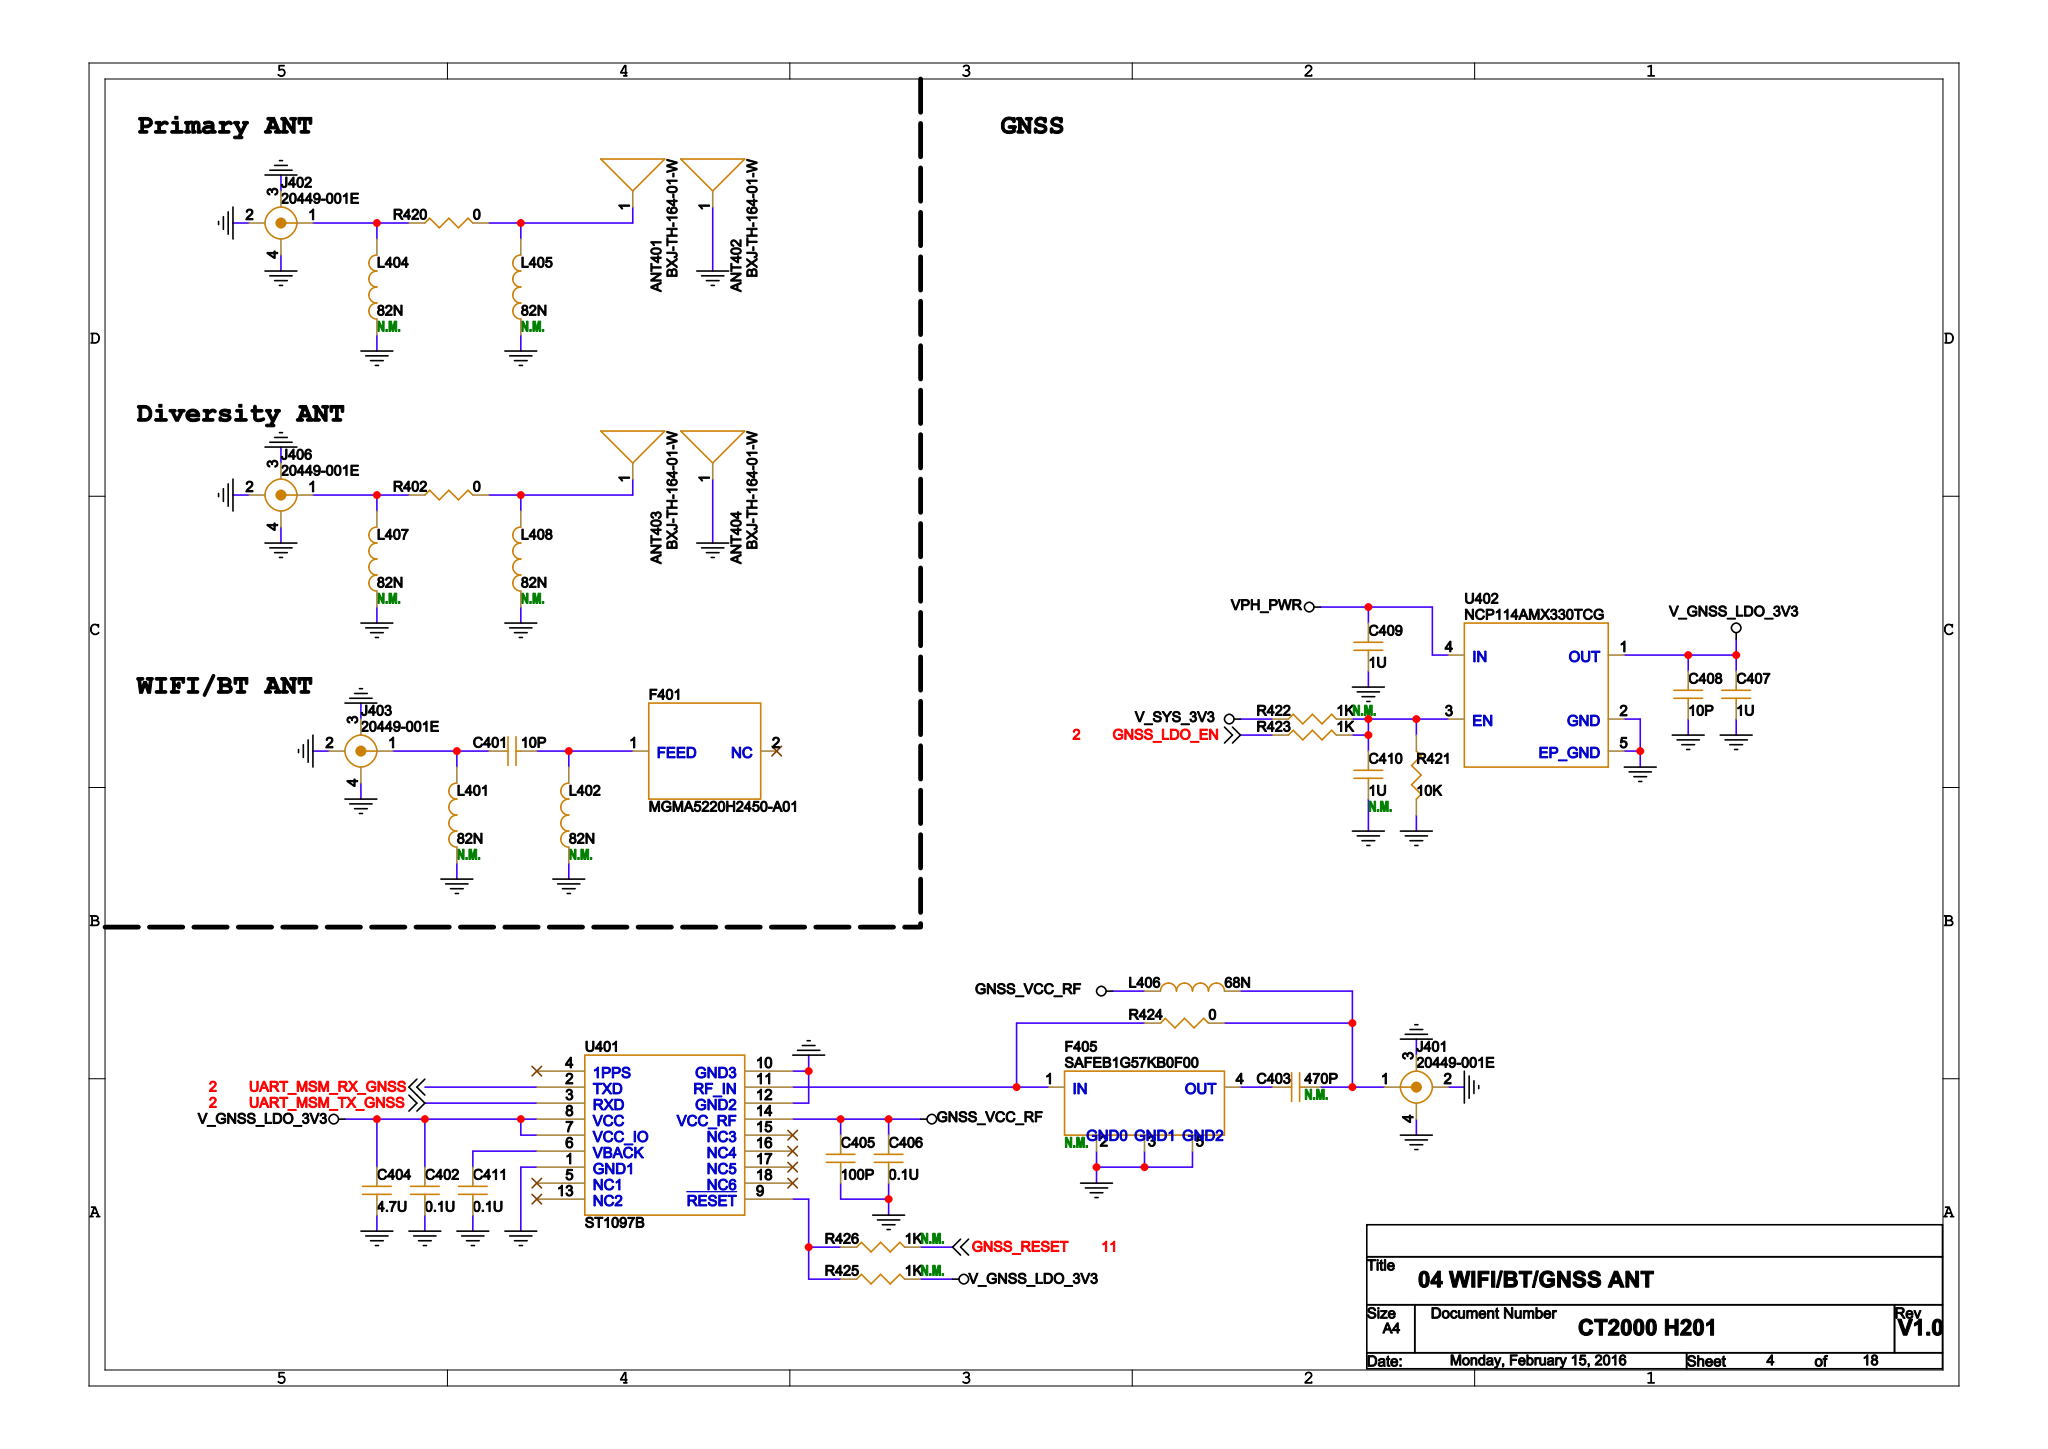Circuit board | Cadence Allegro | 573 parts | 376 nets | one sheet of the schematic
Parts on this sheet (reference | value | footprint):
ANT401 | BXJ-TH-164-01-W | PAD_ANT_BXJ-TH-164-01-W
ANT402 | BXJ-TH-164-01-W | PAD_ANT_BXJ-TH-164-01-W
ANT403 | BXJ-TH-164-01-W | PAD_ANT_BXJ-TH-164-01-W
ANT404 | BXJ-TH-164-01-W | PAD_ANT_BXJ-TH-164-01-W
C401 | 10P | C0402
C402 | 0.1U | C0402
C403 | 470P | C0402
C404 | 4.7U | C0603
C405 | 100P | C0402
C406 | 0.1U | C0402
C407 | 1U | C0402
C408 | 10P | C0402
C409 | 1U | C0402
C410 | 1U | C0402
C411 | 0.1U | C0402
F401 | MGMA5220H2450-A01 | MGMA5220H2450-A01
F405 | SAFEB1G57KB0F00 | SAFEA1G57KJ0F00
J401 | 20449-001E | ANT_CON_IPEX_20449-001E
J402 | 20449-001E | ANT_CON_IPEX_20449-001E
J403 | 20449-001E | ANT_CON_IPEX_20449-001E
J406 | 20449-001E | ANT_CON_IPEX_20449-001E
L401 | 82N | L0402
L402 | 82N | L0402
L404 | 82N | L0402
L405 | 82N | L0402
L406 | 68N | L0402
L407 | 82N | L0402
L408 | 82N | L0402
R402 | 0 | R0402
R420 | 0 | R0402
R421 | 10K | R0402
R422 | 1K | R0402
R423 | 1K | R0402
R424 | 0 | R0402
R425 | 1K | R0402
R426 | 1K | R0402
U401 | ST1097B | MODULE_ST1097B
U402 | NCP114AMX330TCG | UDFN4_1X1X0P7_0P65
Nets of these parts (net: part-pin ...):
GND: ANT402-1 ANT404-1 C402-2 C404-2 C405-2 C406-2 C407-2 C408-2 C409-2 C410-2 C411-2 F405-2 F405-3 F405-5 J401-2 J401-3 J401-4 J402-2 J402-3 J402-4 J403-2 J403-3 J403-4 J406-2 J406-3 J406-4 L401-2 L402-2 L404-2 L405-2 L407-2 L408-2 R421-2 U401-1 U401-10 U401-12 U402-2 U402-5
N52125971: F405-1 R424-1 U401-11
UART_MSM_TX_GNSS: U401-3
N52386768: R425-1 R426-1 U401-9
UART_MSM_RX_GNSS: U401-2
N52859212: C411-1 U401-6
V_GNSS_LDO_3V3: C402-1 C404-1 C407-1 C408-1 R425-2 U401-7 U401-8 U402-1
GNSS_VCC_RF: C405-1 C406-1 L406-2 U401-14
N52797404: ANT403-1 L408-1 R402-2
N52073978: ANT401-1 L405-1 R420-2
V_SYS_3V3: R422-1
VPH_PWR: C409-1 U402-4
GNSS_LDO_EN: R423-1
GNSS_RESET: R426-2
N52797460: J406-1 L407-1 R402-1
N51903323: C403-2 J401-1 L406-1 R424-2
N52073498: J402-1 L404-1 R420-1
N34910168: C401-1 J403-1 L401-1
N51906539: C403-1 F405-4
N34916629: C401-2 F401-1 L402-1
N52126036: C410-1 R421-1 R422-2 R423-2 U402-3